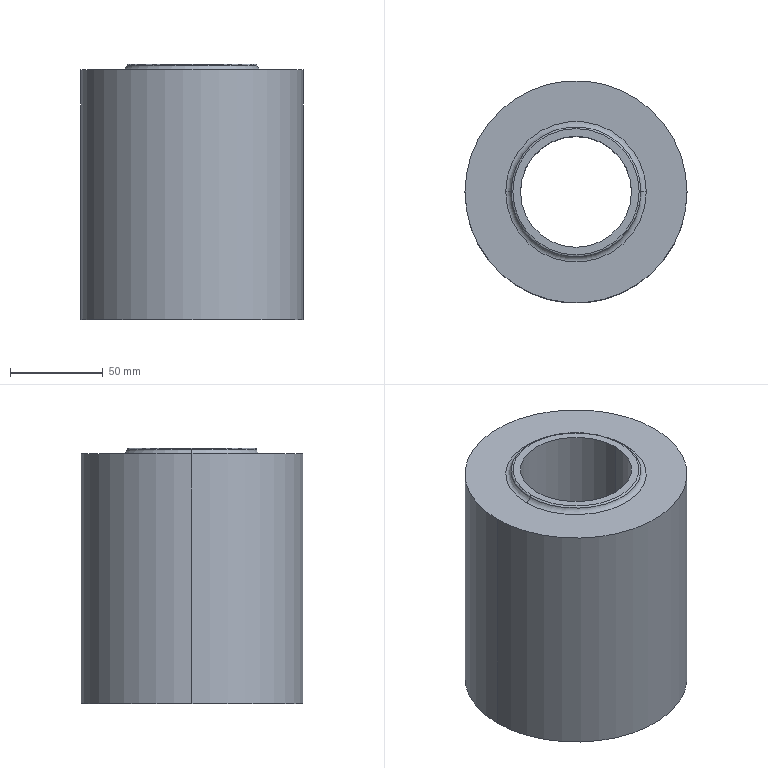Part | SolidWorks | features Fillet 2, Extrusion 1, ICE 1 | 1 solid | 11 faces | box 120 x 120 x 138 mm | volume 1148576 mm3 | torus 4 | cylinder 4 | plane 3 | commonest cylinder face diameters 60 x2 120 x2
STEP:
#1=CARTESIAN_POINT('',(-565.757,0.,3.));
#2=VERTEX_POINT('',#1);
#3=CARTESIAN_POINT('',(-634.011,0.,3.));
#4=VERTEX_POINT('',#3);
#5=CARTESIAN_POINT('',(-599.884,0.,3.));
#6=DIRECTION('',(0.,0.,1.));
#7=DIRECTION('',(1.,0.,0.));
#8=AXIS2_PLACEMENT_3D('',#5,#6,#7);
#9=CIRCLE('',#8,34.127);
#10=EDGE_CURVE('',#2,#4,#9,.T.);
#11=ORIENTED_EDGE('',*,*,#10,.F.);
#12=CARTESIAN_POINT('',(-564.789,0.,2.25));
#13=VERTEX_POINT('',#12);
#14=CARTESIAN_POINT('',(-565.757,0.,2.));
#15=DIRECTION('',(0.,1.,0.));
#16=DIRECTION('',(-1.,0.,0.));
#17=AXIS2_PLACEMENT_3D('',#14,#15,#16);
#18=CIRCLE('',#17,1.);
#19=EDGE_CURVE('',#2,#13,#18,.T.);
#20=ORIENTED_EDGE('',*,*,#19,.T.);
#21=CARTESIAN_POINT('',(-634.979,0.,2.25));
#22=VERTEX_POINT('',#21);
#23=CARTESIAN_POINT('',(-599.884,0.,2.25));
#24=DIRECTION('',(0.,0.,-1.));
#25=DIRECTION('',(1.,0.,0.));
#26=AXIS2_PLACEMENT_3D('',#23,#24,#25);
#27=CIRCLE('',#26,35.095);
#28=EDGE_CURVE('',#22,#13,#27,.T.);
#29=ORIENTED_EDGE('',*,*,#28,.F.);
#30=CARTESIAN_POINT('',(-634.011,0.,2.));
#31=DIRECTION('',(0.,-1.,0.));
#32=DIRECTION('',(0.,0.,-1.));
#33=AXIS2_PLACEMENT_3D('',#30,#31,#32);
#34=CIRCLE('',#33,1.);
#35=EDGE_CURVE('',#4,#22,#34,.T.);
#36=ORIENTED_EDGE('',*,*,#35,.F.);
#37=EDGE_LOOP('',(#11,#20,#29,#36));
#38=FACE_OUTER_BOUND('',#37,.T.);
#39=CARTESIAN_POINT('',(-599.884,0.,2.));
#40=DIRECTION('',(0.,0.,-1.));
#41=DIRECTION('',(-1.,0.,0.));
#42=AXIS2_PLACEMENT_3D('',#39,#40,#41);
#43=TOROIDAL_SURFACE('',#42,34.127,1.);
#44=ADVANCED_FACE('',(#38),#43,.T.);
#45=CARTESIAN_POINT('',(-599.884,0.,2.25));
#46=DIRECTION('',(0.,0.,-1.));
#47=DIRECTION('',(1.,0.,0.));
#48=AXIS2_PLACEMENT_3D('',#45,#46,#47);
#49=CIRCLE('',#48,35.095);
#50=EDGE_CURVE('',#13,#22,#49,.T.);
#51=ORIENTED_EDGE('',*,*,#50,.T.);
#52=CARTESIAN_POINT('',(-637.884,0.,0.));
#53=VERTEX_POINT('',#52);
#54=CARTESIAN_POINT('',(-637.884,0.,3.));
#55=DIRECTION('',(0.,1.,0.));
#56=DIRECTION('',(-1.,0.,0.));
#57=AXIS2_PLACEMENT_3D('',#54,#55,#56);
#58=CIRCLE('',#57,3.);
#59=EDGE_CURVE('',#22,#53,#58,.T.);
#60=ORIENTED_EDGE('',*,*,#59,.T.);
#61=CARTESIAN_POINT('',(-561.884,0.,0.));
#62=VERTEX_POINT('',#61);
#63=CARTESIAN_POINT('',(-599.884,0.,0.));
#64=DIRECTION('',(0.,0.,-1.));
#65=DIRECTION('',(1.,0.,0.));
#66=AXIS2_PLACEMENT_3D('',#63,#64,#65);
#67=CIRCLE('',#66,38.);
#68=EDGE_CURVE('',#62,#53,#67,.T.);
#69=ORIENTED_EDGE('',*,*,#68,.F.);
#70=CARTESIAN_POINT('',(-561.884,0.,3.));
#71=DIRECTION('',(0.,-1.,0.));
#72=DIRECTION('',(0.,0.,-1.));
#73=AXIS2_PLACEMENT_3D('',#70,#71,#72);
#74=CIRCLE('',#73,3.);
#75=EDGE_CURVE('',#13,#62,#74,.T.);
#76=ORIENTED_EDGE('',*,*,#75,.F.);
#77=EDGE_LOOP('',(#51,#60,#69,#76));
#78=FACE_OUTER_BOUND('',#77,.T.);
#79=CARTESIAN_POINT('',(-599.884,0.,3.));
#80=DIRECTION('',(0.,0.,1.));
#81=DIRECTION('',(1.,0.,0.));
#82=AXIS2_PLACEMENT_3D('',#79,#80,#81);
#83=TOROIDAL_SURFACE('',#82,38.,3.);
#84=ADVANCED_FACE('',(#78),#83,.F.);
#85=CARTESIAN_POINT('',(-629.884,0.,-135.));
#86=VERTEX_POINT('',#85);
#87=CARTESIAN_POINT('',(-569.884,0.,-135.));
#88=VERTEX_POINT('',#87);
#89=CARTESIAN_POINT('',(-599.884,0.,-135.));
#90=DIRECTION('',(0.,0.,1.));
#91=DIRECTION('',(1.,0.,0.));
#92=AXIS2_PLACEMENT_3D('',#89,#90,#91);
#93=CIRCLE('',#92,30.);
#94=EDGE_CURVE('',#86,#88,#93,.T.);
#95=ORIENTED_EDGE('',*,*,#94,.F.);
#96=CARTESIAN_POINT('',(-629.884,0.,3.));
#97=VERTEX_POINT('',#96);
#98=CARTESIAN_POINT('',(-629.884,0.,-135.));
#99=DIRECTION('',(0.,0.,1.));
#100=VECTOR('',#99,1000.);
#101=LINE('',#98,#100);
#102=EDGE_CURVE('',#86,#97,#101,.T.);
#103=ORIENTED_EDGE('',*,*,#102,.T.);
#104=CARTESIAN_POINT('',(-569.884,0.,3.));
#105=VERTEX_POINT('',#104);
#106=CARTESIAN_POINT('',(-599.884,0.,3.));
#107=DIRECTION('',(0.,0.,1.));
#108=DIRECTION('',(1.,0.,0.));
#109=AXIS2_PLACEMENT_3D('',#106,#107,#108);
#110=CIRCLE('',#109,30.);
#111=EDGE_CURVE('',#97,#105,#110,.T.);
#112=ORIENTED_EDGE('',*,*,#111,.T.);
#113=CARTESIAN_POINT('',(-569.884,0.,-135.));
#114=DIRECTION('',(0.,0.,1.));
#115=VECTOR('',#114,1000.);
#116=LINE('',#113,#115);
#117=EDGE_CURVE('',#88,#105,#116,.T.);
#118=ORIENTED_EDGE('',*,*,#117,.F.);
#119=EDGE_LOOP('',(#95,#103,#112,#118));
#120=FACE_OUTER_BOUND('',#119,.T.);
#121=CARTESIAN_POINT('',(-599.884,0.,-135.));
#122=DIRECTION('',(0.,0.,1.));
#123=DIRECTION('',(1.,0.,0.));
#124=AXIS2_PLACEMENT_3D('',#121,#122,#123);
#125=CYLINDRICAL_SURFACE('',#124,30.);
#126=ADVANCED_FACE('',(#120),#125,.F.);
#127=CARTESIAN_POINT('',(-539.884,0.,-135.));
#128=VERTEX_POINT('',#127);
#129=CARTESIAN_POINT('',(-659.884,0.,-135.));
#130=VERTEX_POINT('',#129);
#131=CARTESIAN_POINT('',(-599.884,0.,-135.));
#132=DIRECTION('',(0.,0.,1.));
#133=DIRECTION('',(1.,0.,0.));
#134=AXIS2_PLACEMENT_3D('',#131,#132,#133);
#135=CIRCLE('',#134,60.);
#136=EDGE_CURVE('',#128,#130,#135,.T.);
#137=ORIENTED_EDGE('',*,*,#136,.T.);
#138=CARTESIAN_POINT('',(-659.884,0.,0.));
#139=VERTEX_POINT('',#138);
#140=CARTESIAN_POINT('',(-659.884,0.,-135.));
#141=DIRECTION('',(0.,0.,1.));
#142=VECTOR('',#141,1000.);
#143=LINE('',#140,#142);
#144=EDGE_CURVE('',#130,#139,#143,.T.);
#145=ORIENTED_EDGE('',*,*,#144,.T.);
#146=CARTESIAN_POINT('',(-539.884,0.,0.));
#147=VERTEX_POINT('',#146);
#148=CARTESIAN_POINT('',(-599.884,0.,0.));
#149=DIRECTION('',(0.,0.,1.));
#150=DIRECTION('',(1.,0.,0.));
#151=AXIS2_PLACEMENT_3D('',#148,#149,#150);
#152=CIRCLE('',#151,60.);
#153=EDGE_CURVE('',#147,#139,#152,.T.);
#154=ORIENTED_EDGE('',*,*,#153,.F.);
#155=CARTESIAN_POINT('',(-539.884,0.,-135.));
#156=DIRECTION('',(0.,0.,1.));
#157=VECTOR('',#156,1000.);
#158=LINE('',#155,#157);
#159=EDGE_CURVE('',#128,#147,#158,.T.);
#160=ORIENTED_EDGE('',*,*,#159,.F.);
#161=EDGE_LOOP('',(#137,#145,#154,#160));
#162=FACE_OUTER_BOUND('',#161,.T.);
#163=CARTESIAN_POINT('',(-599.884,0.,-135.));
#164=DIRECTION('',(0.,0.,1.));
#165=DIRECTION('',(1.,0.,0.));
#166=AXIS2_PLACEMENT_3D('',#163,#164,#165);
#167=CYLINDRICAL_SURFACE('',#166,60.);
#168=ADVANCED_FACE('',(#162),#167,.T.);
#169=ORIENTED_EDGE('',*,*,#68,.T.);
#170=CARTESIAN_POINT('',(-599.884,0.,0.));
#171=DIRECTION('',(0.,0.,-1.));
#172=DIRECTION('',(1.,0.,0.));
#173=AXIS2_PLACEMENT_3D('',#170,#171,#172);
#174=CIRCLE('',#173,38.);
#175=EDGE_CURVE('',#53,#62,#174,.T.);
#176=ORIENTED_EDGE('',*,*,#175,.T.);
#177=EDGE_LOOP('',(#169,#176));
#178=FACE_BOUND('',#177,.T.);
#179=ORIENTED_EDGE('',*,*,#153,.T.);
#180=CARTESIAN_POINT('',(-599.884,0.,0.));
#181=DIRECTION('',(0.,0.,1.));
#182=DIRECTION('',(1.,0.,0.));
#183=AXIS2_PLACEMENT_3D('',#180,#181,#182);
#184=CIRCLE('',#183,60.);
#185=EDGE_CURVE('',#139,#147,#184,.T.);
#186=ORIENTED_EDGE('',*,*,#185,.T.);
#187=EDGE_LOOP('',(#179,#186));
#188=FACE_OUTER_BOUND('',#187,.T.);
#189=CARTESIAN_POINT('',(-599.884,0.,0.));
#190=DIRECTION('',(0.,0.,1.));
#191=DIRECTION('',(1.,0.,0.));
#192=AXIS2_PLACEMENT_3D('',#189,#190,#191);
#193=PLANE('',#192);
#194=ADVANCED_FACE('',(#178,#188),#193,.T.);
#195=ORIENTED_EDGE('',*,*,#144,.F.);
#196=CARTESIAN_POINT('',(-599.884,0.,-135.));
#197=DIRECTION('',(0.,0.,1.));
#198=DIRECTION('',(1.,0.,0.));
#199=AXIS2_PLACEMENT_3D('',#196,#197,#198);
#200=CIRCLE('',#199,60.);
#201=EDGE_CURVE('',#130,#128,#200,.T.);
#202=ORIENTED_EDGE('',*,*,#201,.T.);
#203=ORIENTED_EDGE('',*,*,#159,.T.);
#204=ORIENTED_EDGE('',*,*,#185,.F.);
#205=EDGE_LOOP('',(#195,#202,#203,#204));
#206=FACE_OUTER_BOUND('',#205,.T.);
#207=CARTESIAN_POINT('',(-599.884,0.,-135.));
#208=DIRECTION('',(0.,0.,1.));
#209=DIRECTION('',(1.,0.,0.));
#210=AXIS2_PLACEMENT_3D('',#207,#208,#209);
#211=CYLINDRICAL_SURFACE('',#210,60.);
#212=ADVANCED_FACE('',(#206),#211,.T.);
#213=CARTESIAN_POINT('',(-599.884,0.,-135.));
#214=DIRECTION('',(0.,0.,1.));
#215=DIRECTION('',(1.,0.,0.));
#216=AXIS2_PLACEMENT_3D('',#213,#214,#215);
#217=CIRCLE('',#216,30.);
#218=EDGE_CURVE('',#88,#86,#217,.T.);
#219=ORIENTED_EDGE('',*,*,#218,.T.);
#220=ORIENTED_EDGE('',*,*,#94,.T.);
#221=EDGE_LOOP('',(#219,#220));
#222=FACE_BOUND('',#221,.T.);
#223=ORIENTED_EDGE('',*,*,#136,.F.);
#224=ORIENTED_EDGE('',*,*,#201,.F.);
#225=EDGE_LOOP('',(#223,#224));
#226=FACE_OUTER_BOUND('',#225,.T.);
#227=CARTESIAN_POINT('',(-599.884,0.,-135.));
#228=DIRECTION('',(0.,0.,1.));
#229=DIRECTION('',(1.,0.,0.));
#230=AXIS2_PLACEMENT_3D('',#227,#228,#229);
#231=PLANE('',#230);
#232=ADVANCED_FACE('',(#222,#226),#231,.F.);
#233=ORIENTED_EDGE('',*,*,#102,.F.);
#234=ORIENTED_EDGE('',*,*,#218,.F.);
#235=ORIENTED_EDGE('',*,*,#117,.T.);
#236=CARTESIAN_POINT('',(-599.884,0.,3.));
#237=DIRECTION('',(0.,0.,1.));
#238=DIRECTION('',(1.,0.,0.));
#239=AXIS2_PLACEMENT_3D('',#236,#237,#238);
#240=CIRCLE('',#239,30.);
#241=EDGE_CURVE('',#105,#97,#240,.T.);
#242=ORIENTED_EDGE('',*,*,#241,.T.);
#243=EDGE_LOOP('',(#233,#234,#235,#242));
#244=FACE_OUTER_BOUND('',#243,.T.);
#245=CARTESIAN_POINT('',(-599.884,0.,-135.));
#246=DIRECTION('',(0.,0.,1.));
#247=DIRECTION('',(1.,0.,0.));
#248=AXIS2_PLACEMENT_3D('',#245,#246,#247);
#249=CYLINDRICAL_SURFACE('',#248,30.);
#250=ADVANCED_FACE('',(#244),#249,.F.);
#251=CARTESIAN_POINT('',(-599.884,0.,3.));
#252=DIRECTION('',(0.,0.,1.));
#253=DIRECTION('',(1.,0.,0.));
#254=AXIS2_PLACEMENT_3D('',#251,#252,#253);
#255=CIRCLE('',#254,34.127);
#256=EDGE_CURVE('',#4,#2,#255,.T.);
#257=ORIENTED_EDGE('',*,*,#256,.T.);
#258=ORIENTED_EDGE('',*,*,#10,.T.);
#259=EDGE_LOOP('',(#257,#258));
#260=FACE_OUTER_BOUND('',#259,.T.);
#261=ORIENTED_EDGE('',*,*,#241,.F.);
#262=ORIENTED_EDGE('',*,*,#111,.F.);
#263=EDGE_LOOP('',(#261,#262));
#264=FACE_BOUND('',#263,.T.);
#265=CARTESIAN_POINT('',(-599.884,0.,3.));
#266=DIRECTION('',(0.,0.,1.));
#267=DIRECTION('',(1.,0.,0.));
#268=AXIS2_PLACEMENT_3D('',#265,#266,#267);
#269=PLANE('',#268);
#270=ADVANCED_FACE('',(#260,#264),#269,.T.);
#271=ORIENTED_EDGE('',*,*,#59,.F.);
#272=ORIENTED_EDGE('',*,*,#28,.T.);
#273=ORIENTED_EDGE('',*,*,#75,.T.);
#274=ORIENTED_EDGE('',*,*,#175,.F.);
#275=EDGE_LOOP('',(#271,#272,#273,#274));
#276=FACE_OUTER_BOUND('',#275,.T.);
#277=CARTESIAN_POINT('',(-599.884,0.,3.));
#278=DIRECTION('',(0.,0.,1.));
#279=DIRECTION('',(1.,0.,0.));
#280=AXIS2_PLACEMENT_3D('',#277,#278,#279);
#281=TOROIDAL_SURFACE('',#280,38.,3.);
#282=ADVANCED_FACE('',(#276),#281,.F.);
#283=ORIENTED_EDGE('',*,*,#19,.F.);
#284=ORIENTED_EDGE('',*,*,#256,.F.);
#285=ORIENTED_EDGE('',*,*,#35,.T.);
#286=ORIENTED_EDGE('',*,*,#50,.F.);
#287=EDGE_LOOP('',(#283,#284,#285,#286));
#288=FACE_OUTER_BOUND('',#287,.T.);
#289=CARTESIAN_POINT('',(-599.884,0.,2.));
#290=DIRECTION('',(0.,0.,-1.));
#291=DIRECTION('',(-1.,0.,0.));
#292=AXIS2_PLACEMENT_3D('',#289,#290,#291);
#293=TOROIDAL_SURFACE('',#292,34.127,1.);
#294=ADVANCED_FACE('',(#288),#293,.T.);
#295=CLOSED_SHELL('',(#44,#84,#126,#168,#194,#212,#232,#250,#270,#282,#294));
#296=MANIFOLD_SOLID_BREP('',#295);
#297=CARTESIAN_POINT('',(0.,0.,0.));
#298=DIRECTION('',(0.,0.,1.));
#299=DIRECTION('',(1.,0.,0.));
#300=AXIS2_PLACEMENT_3D('',#297,#298,#299);
#301=(LENGTH_UNIT()NAMED_UNIT(*)SI_UNIT(.MILLI.,.METRE.));
#302=UNCERTAINTY_MEASURE_WITH_UNIT(LENGTH_MEASURE(0.00001),#301,'','');
#303=(NAMED_UNIT(*)PLANE_ANGLE_UNIT()SI_UNIT($,.RADIAN.));
#304=(NAMED_UNIT(*)SI_UNIT($,.STERADIAN.)SOLID_ANGLE_UNIT());
#305=(GEOMETRIC_REPRESENTATION_CONTEXT(3)GLOBAL_UNCERTAINTY_ASSIGNED_CONTEXT((#302))GLOBAL_UNIT_ASSIGNED_CONTEXT((#301,#303,#304))REPRESENTATION_CONTEXT('',''));
#306=ADVANCED_BREP_SHAPE_REPRESENTATION('',(#296,#300),#305);